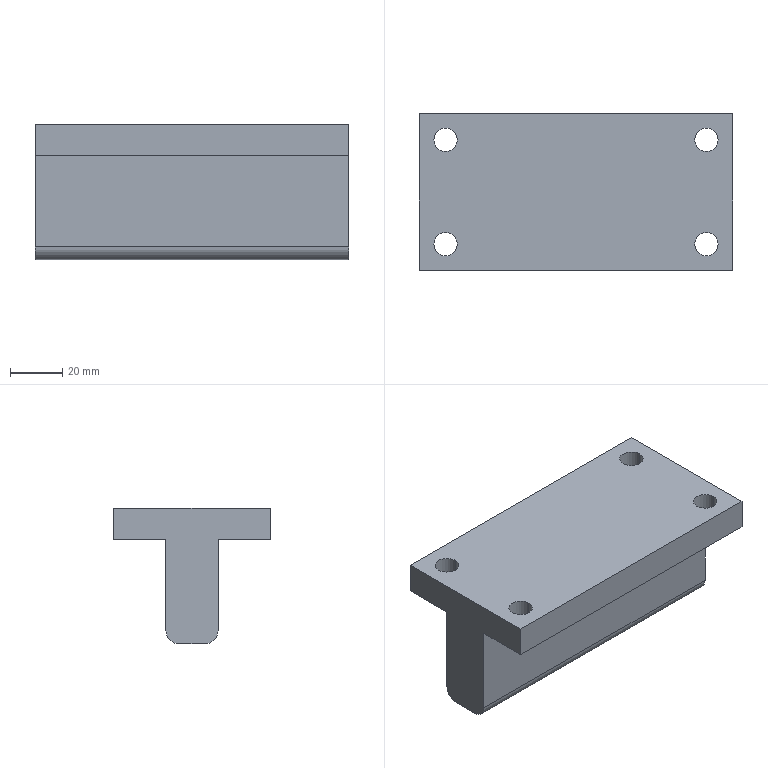Part | SolidWorks | features Extrusion 1, Fillet 1, HoleWzd 1, ICE 1 | 1 solid | 20 faces | box 120 x 60 x 52 mm | volume 178059 mm3 | cylinder 10 | plane 10 | commonest cylinder face diameters 9 x8 10 x2
STEP:
#1=CARTESIAN_POINT('',(114.5,50.,12.));
#2=VERTEX_POINT('',#1);
#3=CARTESIAN_POINT('',(105.5,50.,12.));
#4=VERTEX_POINT('',#3);
#5=CARTESIAN_POINT('',(110.,50.,12.));
#6=DIRECTION('',(0.,0.,-1.));
#7=DIRECTION('',(-1.,0.,0.));
#8=AXIS2_PLACEMENT_3D('',#5,#6,#7);
#9=CIRCLE('',#8,4.5);
#10=EDGE_CURVE('',#2,#4,#9,.T.);
#11=ORIENTED_EDGE('',*,*,#10,.F.);
#12=CARTESIAN_POINT('',(114.5,50.,0.));
#13=VERTEX_POINT('',#12);
#14=CARTESIAN_POINT('',(114.5,50.,0.));
#15=DIRECTION('',(0.,0.,-1.));
#16=VECTOR('',#15,1000.);
#17=LINE('',#14,#16);
#18=EDGE_CURVE('',#2,#13,#17,.T.);
#19=ORIENTED_EDGE('',*,*,#18,.T.);
#20=CARTESIAN_POINT('',(105.5,50.,0.));
#21=VERTEX_POINT('',#20);
#22=CARTESIAN_POINT('',(110.,50.,0.));
#23=DIRECTION('',(0.,0.,-1.));
#24=DIRECTION('',(-1.,0.,0.));
#25=AXIS2_PLACEMENT_3D('',#22,#23,#24);
#26=CIRCLE('',#25,4.5);
#27=EDGE_CURVE('',#13,#21,#26,.T.);
#28=ORIENTED_EDGE('',*,*,#27,.T.);
#29=CARTESIAN_POINT('',(105.5,50.,0.));
#30=DIRECTION('',(0.,0.,-1.));
#31=VECTOR('',#30,1000.);
#32=LINE('',#29,#31);
#33=EDGE_CURVE('',#4,#21,#32,.T.);
#34=ORIENTED_EDGE('',*,*,#33,.F.);
#35=EDGE_LOOP('',(#11,#19,#28,#34));
#36=FACE_OUTER_BOUND('',#35,.T.);
#37=CARTESIAN_POINT('',(110.,50.,0.));
#38=DIRECTION('',(0.,0.,-1.));
#39=DIRECTION('',(-1.,0.,0.));
#40=AXIS2_PLACEMENT_3D('',#37,#38,#39);
#41=CYLINDRICAL_SURFACE('',#40,4.5);
#42=ADVANCED_FACE('',(#36),#41,.F.);
#43=CARTESIAN_POINT('',(14.5,50.,12.));
#44=VERTEX_POINT('',#43);
#45=CARTESIAN_POINT('',(5.5,50.,12.));
#46=VERTEX_POINT('',#45);
#47=CARTESIAN_POINT('',(10.,50.,12.));
#48=DIRECTION('',(0.,0.,-1.));
#49=DIRECTION('',(-1.,0.,0.));
#50=AXIS2_PLACEMENT_3D('',#47,#48,#49);
#51=CIRCLE('',#50,4.5);
#52=EDGE_CURVE('',#44,#46,#51,.T.);
#53=ORIENTED_EDGE('',*,*,#52,.F.);
#54=CARTESIAN_POINT('',(14.5,50.,0.));
#55=VERTEX_POINT('',#54);
#56=CARTESIAN_POINT('',(14.5,50.,0.));
#57=DIRECTION('',(0.,0.,-1.));
#58=VECTOR('',#57,1000.);
#59=LINE('',#56,#58);
#60=EDGE_CURVE('',#44,#55,#59,.T.);
#61=ORIENTED_EDGE('',*,*,#60,.T.);
#62=CARTESIAN_POINT('',(5.5,50.,0.));
#63=VERTEX_POINT('',#62);
#64=CARTESIAN_POINT('',(10.,50.,0.));
#65=DIRECTION('',(0.,0.,-1.));
#66=DIRECTION('',(-1.,0.,0.));
#67=AXIS2_PLACEMENT_3D('',#64,#65,#66);
#68=CIRCLE('',#67,4.5);
#69=EDGE_CURVE('',#55,#63,#68,.T.);
#70=ORIENTED_EDGE('',*,*,#69,.T.);
#71=CARTESIAN_POINT('',(5.5,50.,0.));
#72=DIRECTION('',(0.,0.,-1.));
#73=VECTOR('',#72,1000.);
#74=LINE('',#71,#73);
#75=EDGE_CURVE('',#46,#63,#74,.T.);
#76=ORIENTED_EDGE('',*,*,#75,.F.);
#77=EDGE_LOOP('',(#53,#61,#70,#76));
#78=FACE_OUTER_BOUND('',#77,.T.);
#79=CARTESIAN_POINT('',(10.,50.,0.));
#80=DIRECTION('',(0.,0.,-1.));
#81=DIRECTION('',(-1.,0.,0.));
#82=AXIS2_PLACEMENT_3D('',#79,#80,#81);
#83=CYLINDRICAL_SURFACE('',#82,4.5);
#84=ADVANCED_FACE('',(#78),#83,.F.);
#85=CARTESIAN_POINT('',(14.5,10.,12.));
#86=VERTEX_POINT('',#85);
#87=CARTESIAN_POINT('',(5.5,10.,12.));
#88=VERTEX_POINT('',#87);
#89=CARTESIAN_POINT('',(10.,10.,12.));
#90=DIRECTION('',(0.,0.,-1.));
#91=DIRECTION('',(-1.,0.,0.));
#92=AXIS2_PLACEMENT_3D('',#89,#90,#91);
#93=CIRCLE('',#92,4.5);
#94=EDGE_CURVE('',#86,#88,#93,.T.);
#95=ORIENTED_EDGE('',*,*,#94,.F.);
#96=CARTESIAN_POINT('',(14.5,10.,0.));
#97=VERTEX_POINT('',#96);
#98=CARTESIAN_POINT('',(14.5,10.,0.));
#99=DIRECTION('',(0.,0.,-1.));
#100=VECTOR('',#99,1000.);
#101=LINE('',#98,#100);
#102=EDGE_CURVE('',#86,#97,#101,.T.);
#103=ORIENTED_EDGE('',*,*,#102,.T.);
#104=CARTESIAN_POINT('',(5.5,10.,0.));
#105=VERTEX_POINT('',#104);
#106=CARTESIAN_POINT('',(10.,10.,0.));
#107=DIRECTION('',(0.,0.,-1.));
#108=DIRECTION('',(-1.,0.,0.));
#109=AXIS2_PLACEMENT_3D('',#106,#107,#108);
#110=CIRCLE('',#109,4.5);
#111=EDGE_CURVE('',#97,#105,#110,.T.);
#112=ORIENTED_EDGE('',*,*,#111,.T.);
#113=CARTESIAN_POINT('',(5.5,10.,0.));
#114=DIRECTION('',(0.,0.,-1.));
#115=VECTOR('',#114,1000.);
#116=LINE('',#113,#115);
#117=EDGE_CURVE('',#88,#105,#116,.T.);
#118=ORIENTED_EDGE('',*,*,#117,.F.);
#119=EDGE_LOOP('',(#95,#103,#112,#118));
#120=FACE_OUTER_BOUND('',#119,.T.);
#121=CARTESIAN_POINT('',(10.,10.,0.));
#122=DIRECTION('',(0.,0.,-1.));
#123=DIRECTION('',(-1.,0.,0.));
#124=AXIS2_PLACEMENT_3D('',#121,#122,#123);
#125=CYLINDRICAL_SURFACE('',#124,4.5);
#126=ADVANCED_FACE('',(#120),#125,.F.);
#127=CARTESIAN_POINT('',(114.5,10.,12.));
#128=VERTEX_POINT('',#127);
#129=CARTESIAN_POINT('',(105.5,10.,12.));
#130=VERTEX_POINT('',#129);
#131=CARTESIAN_POINT('',(110.,10.,12.));
#132=DIRECTION('',(0.,0.,-1.));
#133=DIRECTION('',(-1.,0.,0.));
#134=AXIS2_PLACEMENT_3D('',#131,#132,#133);
#135=CIRCLE('',#134,4.5);
#136=EDGE_CURVE('',#128,#130,#135,.T.);
#137=ORIENTED_EDGE('',*,*,#136,.F.);
#138=CARTESIAN_POINT('',(114.5,10.,0.));
#139=VERTEX_POINT('',#138);
#140=CARTESIAN_POINT('',(114.5,10.,0.));
#141=DIRECTION('',(0.,0.,-1.));
#142=VECTOR('',#141,1000.);
#143=LINE('',#140,#142);
#144=EDGE_CURVE('',#128,#139,#143,.T.);
#145=ORIENTED_EDGE('',*,*,#144,.T.);
#146=CARTESIAN_POINT('',(105.5,10.,0.));
#147=VERTEX_POINT('',#146);
#148=CARTESIAN_POINT('',(110.,10.,0.));
#149=DIRECTION('',(0.,0.,-1.));
#150=DIRECTION('',(-1.,0.,0.));
#151=AXIS2_PLACEMENT_3D('',#148,#149,#150);
#152=CIRCLE('',#151,4.5);
#153=EDGE_CURVE('',#139,#147,#152,.T.);
#154=ORIENTED_EDGE('',*,*,#153,.T.);
#155=CARTESIAN_POINT('',(105.5,10.,0.));
#156=DIRECTION('',(0.,0.,-1.));
#157=VECTOR('',#156,1000.);
#158=LINE('',#155,#157);
#159=EDGE_CURVE('',#130,#147,#158,.T.);
#160=ORIENTED_EDGE('',*,*,#159,.F.);
#161=EDGE_LOOP('',(#137,#145,#154,#160));
#162=FACE_OUTER_BOUND('',#161,.T.);
#163=CARTESIAN_POINT('',(110.,10.,0.));
#164=DIRECTION('',(0.,0.,-1.));
#165=DIRECTION('',(-1.,0.,0.));
#166=AXIS2_PLACEMENT_3D('',#163,#164,#165);
#167=CYLINDRICAL_SURFACE('',#166,4.5);
#168=ADVANCED_FACE('',(#162),#167,.F.);
#169=CARTESIAN_POINT('',(110.,50.,0.));
#170=DIRECTION('',(0.,0.,-1.));
#171=DIRECTION('',(-1.,0.,0.));
#172=AXIS2_PLACEMENT_3D('',#169,#170,#171);
#173=CIRCLE('',#172,4.5);
#174=EDGE_CURVE('',#21,#13,#173,.T.);
#175=ORIENTED_EDGE('',*,*,#174,.F.);
#176=ORIENTED_EDGE('',*,*,#27,.F.);
#177=EDGE_LOOP('',(#175,#176));
#178=FACE_BOUND('',#177,.T.);
#179=CARTESIAN_POINT('',(10.,50.,0.));
#180=DIRECTION('',(0.,0.,-1.));
#181=DIRECTION('',(-1.,0.,0.));
#182=AXIS2_PLACEMENT_3D('',#179,#180,#181);
#183=CIRCLE('',#182,4.5);
#184=EDGE_CURVE('',#63,#55,#183,.T.);
#185=ORIENTED_EDGE('',*,*,#184,.F.);
#186=ORIENTED_EDGE('',*,*,#69,.F.);
#187=EDGE_LOOP('',(#185,#186));
#188=FACE_BOUND('',#187,.T.);
#189=CARTESIAN_POINT('',(120.,40.,0.));
#190=VERTEX_POINT('',#189);
#191=CARTESIAN_POINT('',(120.,60.,0.));
#192=VERTEX_POINT('',#191);
#193=CARTESIAN_POINT('',(120.,0.,0.));
#194=DIRECTION('',(0.,1.,0.));
#195=VECTOR('',#194,1000.);
#196=LINE('',#193,#195);
#197=EDGE_CURVE('',#190,#192,#196,.T.);
#198=ORIENTED_EDGE('',*,*,#197,.F.);
#199=CARTESIAN_POINT('',(0.,40.,0.));
#200=VERTEX_POINT('',#199);
#201=CARTESIAN_POINT('',(0.,40.,0.));
#202=DIRECTION('',(-1.,0.,0.));
#203=VECTOR('',#202,1000.);
#204=LINE('',#201,#203);
#205=EDGE_CURVE('',#190,#200,#204,.T.);
#206=ORIENTED_EDGE('',*,*,#205,.T.);
#207=CARTESIAN_POINT('',(0.,60.,0.));
#208=VERTEX_POINT('',#207);
#209=CARTESIAN_POINT('',(0.,0.,0.));
#210=DIRECTION('',(0.,1.,0.));
#211=VECTOR('',#210,1000.);
#212=LINE('',#209,#211);
#213=EDGE_CURVE('',#200,#208,#212,.T.);
#214=ORIENTED_EDGE('',*,*,#213,.T.);
#215=CARTESIAN_POINT('',(0.,60.,0.));
#216=DIRECTION('',(1.,0.,0.));
#217=VECTOR('',#216,1000.);
#218=LINE('',#215,#217);
#219=EDGE_CURVE('',#208,#192,#218,.T.);
#220=ORIENTED_EDGE('',*,*,#219,.T.);
#221=EDGE_LOOP('',(#198,#206,#214,#220));
#222=FACE_OUTER_BOUND('',#221,.T.);
#223=CARTESIAN_POINT('',(0.,0.,0.));
#224=DIRECTION('',(0.,0.,-1.));
#225=DIRECTION('',(-1.,0.,0.));
#226=AXIS2_PLACEMENT_3D('',#223,#224,#225);
#227=PLANE('',#226);
#228=ADVANCED_FACE('',(#178,#188,#222),#227,.T.);
#229=CARTESIAN_POINT('',(110.,10.,0.));
#230=DIRECTION('',(0.,0.,-1.));
#231=DIRECTION('',(-1.,0.,0.));
#232=AXIS2_PLACEMENT_3D('',#229,#230,#231);
#233=CIRCLE('',#232,4.5);
#234=EDGE_CURVE('',#147,#139,#233,.T.);
#235=ORIENTED_EDGE('',*,*,#234,.F.);
#236=ORIENTED_EDGE('',*,*,#153,.F.);
#237=EDGE_LOOP('',(#235,#236));
#238=FACE_BOUND('',#237,.T.);
#239=CARTESIAN_POINT('',(10.,10.,0.));
#240=DIRECTION('',(0.,0.,-1.));
#241=DIRECTION('',(-1.,0.,0.));
#242=AXIS2_PLACEMENT_3D('',#239,#240,#241);
#243=CIRCLE('',#242,4.5);
#244=EDGE_CURVE('',#105,#97,#243,.T.);
#245=ORIENTED_EDGE('',*,*,#244,.F.);
#246=ORIENTED_EDGE('',*,*,#111,.F.);
#247=EDGE_LOOP('',(#245,#246));
#248=FACE_BOUND('',#247,.T.);
#249=CARTESIAN_POINT('',(0.,0.,0.));
#250=VERTEX_POINT('',#249);
#251=CARTESIAN_POINT('',(0.,20.,0.));
#252=VERTEX_POINT('',#251);
#253=CARTESIAN_POINT('',(0.,0.,0.));
#254=DIRECTION('',(0.,1.,0.));
#255=VECTOR('',#254,1000.);
#256=LINE('',#253,#255);
#257=EDGE_CURVE('',#250,#252,#256,.T.);
#258=ORIENTED_EDGE('',*,*,#257,.T.);
#259=CARTESIAN_POINT('',(120.,20.,0.));
#260=VERTEX_POINT('',#259);
#261=CARTESIAN_POINT('',(0.,20.,0.));
#262=DIRECTION('',(1.,0.,0.));
#263=VECTOR('',#262,1000.);
#264=LINE('',#261,#263);
#265=EDGE_CURVE('',#252,#260,#264,.T.);
#266=ORIENTED_EDGE('',*,*,#265,.T.);
#267=CARTESIAN_POINT('',(120.,0.,0.));
#268=VERTEX_POINT('',#267);
#269=CARTESIAN_POINT('',(120.,0.,0.));
#270=DIRECTION('',(0.,1.,0.));
#271=VECTOR('',#270,1000.);
#272=LINE('',#269,#271);
#273=EDGE_CURVE('',#268,#260,#272,.T.);
#274=ORIENTED_EDGE('',*,*,#273,.F.);
#275=CARTESIAN_POINT('',(0.,0.,0.));
#276=DIRECTION('',(1.,0.,0.));
#277=VECTOR('',#276,1000.);
#278=LINE('',#275,#277);
#279=EDGE_CURVE('',#250,#268,#278,.T.);
#280=ORIENTED_EDGE('',*,*,#279,.F.);
#281=EDGE_LOOP('',(#258,#266,#274,#280));
#282=FACE_OUTER_BOUND('',#281,.T.);
#283=CARTESIAN_POINT('',(0.,0.,0.));
#284=DIRECTION('',(0.,0.,-1.));
#285=DIRECTION('',(-1.,0.,0.));
#286=AXIS2_PLACEMENT_3D('',#283,#284,#285);
#287=PLANE('',#286);
#288=ADVANCED_FACE('',(#238,#248,#282),#287,.T.);
#289=CARTESIAN_POINT('',(0.,40.,-35.));
#290=VERTEX_POINT('',#289);
#291=CARTESIAN_POINT('',(0.,40.,-40.));
#292=DIRECTION('',(0.,0.,1.));
#293=VECTOR('',#292,1000.);
#294=LINE('',#291,#293);
#295=EDGE_CURVE('',#290,#200,#294,.T.);
#296=ORIENTED_EDGE('',*,*,#295,.F.);
#297=CARTESIAN_POINT('',(0.,35.,-40.));
#298=VERTEX_POINT('',#297);
#299=CARTESIAN_POINT('',(0.,35.,-35.));
#300=DIRECTION('',(-1.,0.,0.));
#301=DIRECTION('',(0.,0.,1.));
#302=AXIS2_PLACEMENT_3D('',#299,#300,#301);
#303=CIRCLE('',#302,5.);
#304=EDGE_CURVE('',#290,#298,#303,.T.);
#305=ORIENTED_EDGE('',*,*,#304,.T.);
#306=CARTESIAN_POINT('',(0.,25.,-40.));
#307=VERTEX_POINT('',#306);
#308=CARTESIAN_POINT('',(0.,40.,-40.));
#309=DIRECTION('',(0.,-1.,0.));
#310=VECTOR('',#309,1000.);
#311=LINE('',#308,#310);
#312=EDGE_CURVE('',#298,#307,#311,.T.);
#313=ORIENTED_EDGE('',*,*,#312,.T.);
#314=CARTESIAN_POINT('',(0.,20.,-35.));
#315=VERTEX_POINT('',#314);
#316=CARTESIAN_POINT('',(0.,25.,-35.));
#317=DIRECTION('',(-1.,0.,0.));
#318=DIRECTION('',(0.,0.,1.));
#319=AXIS2_PLACEMENT_3D('',#316,#317,#318);
#320=CIRCLE('',#319,5.);
#321=EDGE_CURVE('',#307,#315,#320,.T.);
#322=ORIENTED_EDGE('',*,*,#321,.T.);
#323=CARTESIAN_POINT('',(0.,20.,-40.));
#324=DIRECTION('',(0.,0.,1.));
#325=VECTOR('',#324,1000.);
#326=LINE('',#323,#325);
#327=EDGE_CURVE('',#315,#252,#326,.T.);
#328=ORIENTED_EDGE('',*,*,#327,.T.);
#329=ORIENTED_EDGE('',*,*,#257,.F.);
#330=CARTESIAN_POINT('',(0.,0.,12.));
#331=VERTEX_POINT('',#330);
#332=CARTESIAN_POINT('',(0.,0.,12.));
#333=DIRECTION('',(0.,0.,-1.));
#334=VECTOR('',#333,1000.);
#335=LINE('',#332,#334);
#336=EDGE_CURVE('',#331,#250,#335,.T.);
#337=ORIENTED_EDGE('',*,*,#336,.F.);
#338=CARTESIAN_POINT('',(0.,60.,12.));
#339=VERTEX_POINT('',#338);
#340=CARTESIAN_POINT('',(0.,0.,12.));
#341=DIRECTION('',(0.,1.,0.));
#342=VECTOR('',#341,1000.);
#343=LINE('',#340,#342);
#344=EDGE_CURVE('',#331,#339,#343,.T.);
#345=ORIENTED_EDGE('',*,*,#344,.T.);
#346=CARTESIAN_POINT('',(0.,60.,12.));
#347=DIRECTION('',(0.,0.,-1.));
#348=VECTOR('',#347,1000.);
#349=LINE('',#346,#348);
#350=EDGE_CURVE('',#339,#208,#349,.T.);
#351=ORIENTED_EDGE('',*,*,#350,.T.);
#352=ORIENTED_EDGE('',*,*,#213,.F.);
#353=EDGE_LOOP('',(#296,#305,#313,#322,#328,#329,#337,#345,#351,#352));
#354=FACE_OUTER_BOUND('',#353,.T.);
#355=CARTESIAN_POINT('',(0.,0.,12.));
#356=DIRECTION('',(-1.,0.,0.));
#357=DIRECTION('',(0.,0.,1.));
#358=AXIS2_PLACEMENT_3D('',#355,#356,#357);
#359=PLANE('',#358);
#360=ADVANCED_FACE('',(#354),#359,.T.);
#361=ORIENTED_EDGE('',*,*,#279,.T.);
#362=CARTESIAN_POINT('',(120.,0.,12.));
#363=VERTEX_POINT('',#362);
#364=CARTESIAN_POINT('',(120.,0.,12.));
#365=DIRECTION('',(0.,0.,-1.));
#366=VECTOR('',#365,1000.);
#367=LINE('',#364,#366);
#368=EDGE_CURVE('',#363,#268,#367,.T.);
#369=ORIENTED_EDGE('',*,*,#368,.F.);
#370=CARTESIAN_POINT('',(0.,0.,12.));
#371=DIRECTION('',(1.,0.,0.));
#372=VECTOR('',#371,1000.);
#373=LINE('',#370,#372);
#374=EDGE_CURVE('',#331,#363,#373,.T.);
#375=ORIENTED_EDGE('',*,*,#374,.F.);
#376=ORIENTED_EDGE('',*,*,#336,.T.);
#377=EDGE_LOOP('',(#361,#369,#375,#376));
#378=FACE_OUTER_BOUND('',#377,.T.);
#379=CARTESIAN_POINT('',(0.,0.,12.));
#380=DIRECTION('',(0.,1.,0.));
#381=DIRECTION('',(0.,0.,1.));
#382=AXIS2_PLACEMENT_3D('',#379,#380,#381);
#383=PLANE('',#382);
#384=ADVANCED_FACE('',(#378),#383,.F.);
#385=CARTESIAN_POINT('',(120.,25.,-40.));
#386=VERTEX_POINT('',#385);
#387=CARTESIAN_POINT('',(120.,35.,-40.));
#388=VERTEX_POINT('',#387);
#389=CARTESIAN_POINT('',(120.,40.,-40.));
#390=DIRECTION('',(0.,1.,0.));
#391=VECTOR('',#390,1000.);
#392=LINE('',#389,#391);
#393=EDGE_CURVE('',#386,#388,#392,.T.);
#394=ORIENTED_EDGE('',*,*,#393,.T.);
#395=CARTESIAN_POINT('',(120.,40.,-35.));
#396=VERTEX_POINT('',#395);
#397=CARTESIAN_POINT('',(120.,35.,-35.));
#398=DIRECTION('',(1.,0.,0.));
#399=DIRECTION('',(0.,0.,1.));
#400=AXIS2_PLACEMENT_3D('',#397,#398,#399);
#401=CIRCLE('',#400,5.);
#402=EDGE_CURVE('',#388,#396,#401,.T.);
#403=ORIENTED_EDGE('',*,*,#402,.T.);
#404=CARTESIAN_POINT('',(120.,40.,-40.));
#405=DIRECTION('',(0.,0.,1.));
#406=VECTOR('',#405,1000.);
#407=LINE('',#404,#406);
#408=EDGE_CURVE('',#396,#190,#407,.T.);
#409=ORIENTED_EDGE('',*,*,#408,.T.);
#410=ORIENTED_EDGE('',*,*,#197,.T.);
#411=CARTESIAN_POINT('',(120.,60.,12.));
#412=VERTEX_POINT('',#411);
#413=CARTESIAN_POINT('',(120.,60.,12.));
#414=DIRECTION('',(0.,0.,-1.));
#415=VECTOR('',#414,1000.);
#416=LINE('',#413,#415);
#417=EDGE_CURVE('',#412,#192,#416,.T.);
#418=ORIENTED_EDGE('',*,*,#417,.F.);
#419=CARTESIAN_POINT('',(120.,0.,12.));
#420=DIRECTION('',(0.,1.,0.));
#421=VECTOR('',#420,1000.);
#422=LINE('',#419,#421);
#423=EDGE_CURVE('',#363,#412,#422,.T.);
#424=ORIENTED_EDGE('',*,*,#423,.F.);
#425=ORIENTED_EDGE('',*,*,#368,.T.);
#426=ORIENTED_EDGE('',*,*,#273,.T.);
#427=CARTESIAN_POINT('',(120.,20.,-35.));
#428=VERTEX_POINT('',#427);
#429=CARTESIAN_POINT('',(120.,20.,-40.));
#430=DIRECTION('',(0.,0.,1.));
#431=VECTOR('',#430,1000.);
#432=LINE('',#429,#431);
#433=EDGE_CURVE('',#428,#260,#432,.T.);
#434=ORIENTED_EDGE('',*,*,#433,.F.);
#435=CARTESIAN_POINT('',(120.,25.,-35.));
#436=DIRECTION('',(1.,0.,0.));
#437=DIRECTION('',(0.,0.,1.));
#438=AXIS2_PLACEMENT_3D('',#435,#436,#437);
#439=CIRCLE('',#438,5.);
#440=EDGE_CURVE('',#428,#386,#439,.T.);
#441=ORIENTED_EDGE('',*,*,#440,.T.);
#442=EDGE_LOOP('',(#394,#403,#409,#410,#418,#424,#425,#426,#434,#441));
#443=FACE_OUTER_BOUND('',#442,.T.);
#444=CARTESIAN_POINT('',(120.,0.,12.));
#445=DIRECTION('',(-1.,0.,0.));
#446=DIRECTION('',(0.,0.,1.));
#447=AXIS2_PLACEMENT_3D('',#444,#445,#446);
#448=PLANE('',#447);
#449=ADVANCED_FACE('',(#443),#448,.F.);
#450=ORIENTED_EDGE('',*,*,#219,.F.);
#451=ORIENTED_EDGE('',*,*,#350,.F.);
#452=CARTESIAN_POINT('',(0.,60.,12.));
#453=DIRECTION('',(1.,0.,0.));
#454=VECTOR('',#453,1000.);
#455=LINE('',#452,#454);
#456=EDGE_CURVE('',#339,#412,#455,.T.);
#457=ORIENTED_EDGE('',*,*,#456,.T.);
#458=ORIENTED_EDGE('',*,*,#417,.T.);
#459=EDGE_LOOP('',(#450,#451,#457,#458));
#460=FACE_OUTER_BOUND('',#459,.T.);
#461=CARTESIAN_POINT('',(0.,60.,12.));
#462=DIRECTION('',(0.,1.,0.));
#463=DIRECTION('',(0.,0.,1.));
#464=AXIS2_PLACEMENT_3D('',#461,#462,#463);
#465=PLANE('',#464);
#466=ADVANCED_FACE('',(#460),#465,.T.);
#467=CARTESIAN_POINT('',(110.,50.,12.));
#468=DIRECTION('',(0.,0.,-1.));
#469=DIRECTION('',(-1.,0.,0.));
#470=AXIS2_PLACEMENT_3D('',#467,#468,#469);
#471=CIRCLE('',#470,4.5);
#472=EDGE_CURVE('',#4,#2,#471,.T.);
#473=ORIENTED_EDGE('',*,*,#472,.T.);
#474=ORIENTED_EDGE('',*,*,#10,.T.);
#475=EDGE_LOOP('',(#473,#474));
#476=FACE_BOUND('',#475,.T.);
#477=CARTESIAN_POINT('',(10.,50.,12.));
#478=DIRECTION('',(0.,0.,-1.));
#479=DIRECTION('',(-1.,0.,0.));
#480=AXIS2_PLACEMENT_3D('',#477,#478,#479);
#481=CIRCLE('',#480,4.5);
#482=EDGE_CURVE('',#46,#44,#481,.T.);
#483=ORIENTED_EDGE('',*,*,#482,.T.);
#484=ORIENTED_EDGE('',*,*,#52,.T.);
#485=EDGE_LOOP('',(#483,#484));
#486=FACE_BOUND('',#485,.T.);
#487=CARTESIAN_POINT('',(10.,10.,12.));
#488=DIRECTION('',(0.,0.,-1.));
#489=DIRECTION('',(-1.,0.,0.));
#490=AXIS2_PLACEMENT_3D('',#487,#488,#489);
#491=CIRCLE('',#490,4.5);
#492=EDGE_CURVE('',#88,#86,#491,.T.);
#493=ORIENTED_EDGE('',*,*,#492,.T.);
#494=ORIENTED_EDGE('',*,*,#94,.T.);
#495=EDGE_LOOP('',(#493,#494));
#496=FACE_BOUND('',#495,.T.);
#497=CARTESIAN_POINT('',(110.,10.,12.));
#498=DIRECTION('',(0.,0.,-1.));
#499=DIRECTION('',(-1.,0.,0.));
#500=AXIS2_PLACEMENT_3D('',#497,#498,#499);
#501=CIRCLE('',#500,4.5);
#502=EDGE_CURVE('',#130,#128,#501,.T.);
#503=ORIENTED_EDGE('',*,*,#502,.T.);
#504=ORIENTED_EDGE('',*,*,#136,.T.);
#505=EDGE_LOOP('',(#503,#504));
#506=FACE_BOUND('',#505,.T.);
#507=ORIENTED_EDGE('',*,*,#344,.F.);
#508=ORIENTED_EDGE('',*,*,#374,.T.);
#509=ORIENTED_EDGE('',*,*,#423,.T.);
#510=ORIENTED_EDGE('',*,*,#456,.F.);
#511=EDGE_LOOP('',(#507,#508,#509,#510));
#512=FACE_OUTER_BOUND('',#511,.T.);
#513=CARTESIAN_POINT('',(0.,0.,12.));
#514=DIRECTION('',(0.,0.,-1.));
#515=DIRECTION('',(-1.,0.,0.));
#516=AXIS2_PLACEMENT_3D('',#513,#514,#515);
#517=PLANE('',#516);
#518=ADVANCED_FACE('',(#476,#486,#496,#506,#512),#517,.F.);
#519=ORIENTED_EDGE('',*,*,#144,.F.);
#520=ORIENTED_EDGE('',*,*,#502,.F.);
#521=ORIENTED_EDGE('',*,*,#159,.T.);
#522=ORIENTED_EDGE('',*,*,#234,.T.);
#523=EDGE_LOOP('',(#519,#520,#521,#522));
#524=FACE_OUTER_BOUND('',#523,.T.);
#525=CARTESIAN_POINT('',(110.,10.,0.));
#526=DIRECTION('',(0.,0.,-1.));
#527=DIRECTION('',(-1.,0.,0.));
#528=AXIS2_PLACEMENT_3D('',#525,#526,#527);
#529=CYLINDRICAL_SURFACE('',#528,4.5);
#530=ADVANCED_FACE('',(#524),#529,.F.);
#531=ORIENTED_EDGE('',*,*,#102,.F.);
#532=ORIENTED_EDGE('',*,*,#492,.F.);
#533=ORIENTED_EDGE('',*,*,#117,.T.);
#534=ORIENTED_EDGE('',*,*,#244,.T.);
#535=EDGE_LOOP('',(#531,#532,#533,#534));
#536=FACE_OUTER_BOUND('',#535,.T.);
#537=CARTESIAN_POINT('',(10.,10.,0.));
#538=DIRECTION('',(0.,0.,-1.));
#539=DIRECTION('',(-1.,0.,0.));
#540=AXIS2_PLACEMENT_3D('',#537,#538,#539);
#541=CYLINDRICAL_SURFACE('',#540,4.5);
#542=ADVANCED_FACE('',(#536),#541,.F.);
#543=ORIENTED_EDGE('',*,*,#60,.F.);
#544=ORIENTED_EDGE('',*,*,#482,.F.);
#545=ORIENTED_EDGE('',*,*,#75,.T.);
#546=ORIENTED_EDGE('',*,*,#184,.T.);
#547=EDGE_LOOP('',(#543,#544,#545,#546));
#548=FACE_OUTER_BOUND('',#547,.T.);
#549=CARTESIAN_POINT('',(10.,50.,0.));
#550=DIRECTION('',(0.,0.,-1.));
#551=DIRECTION('',(-1.,0.,0.));
#552=AXIS2_PLACEMENT_3D('',#549,#550,#551);
#553=CYLINDRICAL_SURFACE('',#552,4.5);
#554=ADVANCED_FACE('',(#548),#553,.F.);
#555=ORIENTED_EDGE('',*,*,#18,.F.);
#556=ORIENTED_EDGE('',*,*,#472,.F.);
#557=ORIENTED_EDGE('',*,*,#33,.T.);
#558=ORIENTED_EDGE('',*,*,#174,.T.);
#559=EDGE_LOOP('',(#555,#556,#557,#558));
#560=FACE_OUTER_BOUND('',#559,.T.);
#561=CARTESIAN_POINT('',(110.,50.,0.));
#562=DIRECTION('',(0.,0.,-1.));
#563=DIRECTION('',(-1.,0.,0.));
#564=AXIS2_PLACEMENT_3D('',#561,#562,#563);
#565=CYLINDRICAL_SURFACE('',#564,4.5);
#566=ADVANCED_FACE('',(#560),#565,.F.);
#567=ORIENTED_EDGE('',*,*,#327,.F.);
#568=CARTESIAN_POINT('',(120.,20.,-35.));
#569=DIRECTION('',(1.,0.,0.));
#570=VECTOR('',#569,1000.);
#571=LINE('',#568,#570);
#572=EDGE_CURVE('',#315,#428,#571,.T.);
#573=ORIENTED_EDGE('',*,*,#572,.T.);
#574=ORIENTED_EDGE('',*,*,#433,.T.);
#575=ORIENTED_EDGE('',*,*,#265,.F.);
#576=EDGE_LOOP('',(#567,#573,#574,#575));
#577=FACE_OUTER_BOUND('',#576,.T.);
#578=CARTESIAN_POINT('',(0.,20.,-40.));
#579=DIRECTION('',(0.,-1.,0.));
#580=DIRECTION('',(0.,0.,-1.));
#581=AXIS2_PLACEMENT_3D('',#578,#579,#580);
#582=PLANE('',#581);
#583=ADVANCED_FACE('',(#577),#582,.T.);
#584=ORIENTED_EDGE('',*,*,#408,.F.);
#585=CARTESIAN_POINT('',(0.,40.,-35.));
#586=DIRECTION('',(-1.,0.,0.));
#587=VECTOR('',#586,1000.);
#588=LINE('',#585,#587);
#589=EDGE_CURVE('',#396,#290,#588,.T.);
#590=ORIENTED_EDGE('',*,*,#589,.T.);
#591=ORIENTED_EDGE('',*,*,#295,.T.);
#592=ORIENTED_EDGE('',*,*,#205,.F.);
#593=EDGE_LOOP('',(#584,#590,#591,#592));
#594=FACE_OUTER_BOUND('',#593,.T.);
#595=CARTESIAN_POINT('',(0.,40.,-40.));
#596=DIRECTION('',(0.,1.,0.));
#597=DIRECTION('',(0.,0.,1.));
#598=AXIS2_PLACEMENT_3D('',#595,#596,#597);
#599=PLANE('',#598);
#600=ADVANCED_FACE('',(#594),#599,.T.);
#601=ORIENTED_EDGE('',*,*,#312,.F.);
#602=CARTESIAN_POINT('',(120.,35.,-40.));
#603=DIRECTION('',(1.,0.,0.));
#604=VECTOR('',#603,1000.);
#605=LINE('',#602,#604);
#606=EDGE_CURVE('',#298,#388,#605,.T.);
#607=ORIENTED_EDGE('',*,*,#606,.T.);
#608=ORIENTED_EDGE('',*,*,#393,.F.);
#609=CARTESIAN_POINT('',(0.,25.,-40.));
#610=DIRECTION('',(-1.,0.,0.));
#611=VECTOR('',#610,1000.);
#612=LINE('',#609,#611);
#613=EDGE_CURVE('',#386,#307,#612,.T.);
#614=ORIENTED_EDGE('',*,*,#613,.T.);
#615=EDGE_LOOP('',(#601,#607,#608,#614));
#616=FACE_OUTER_BOUND('',#615,.T.);
#617=CARTESIAN_POINT('',(0.,0.,-40.));
#618=DIRECTION('',(0.,0.,1.));
#619=DIRECTION('',(1.,0.,0.));
#620=AXIS2_PLACEMENT_3D('',#617,#618,#619);
#621=PLANE('',#620);
#622=ADVANCED_FACE('',(#616),#621,.F.);
#623=ORIENTED_EDGE('',*,*,#402,.F.);
#624=ORIENTED_EDGE('',*,*,#606,.F.);
#625=ORIENTED_EDGE('',*,*,#304,.F.);
#626=ORIENTED_EDGE('',*,*,#589,.F.);
#627=EDGE_LOOP('',(#623,#624,#625,#626));
#628=FACE_OUTER_BOUND('',#627,.T.);
#629=CARTESIAN_POINT('',(0.,35.,-35.));
#630=DIRECTION('',(1.,0.,0.));
#631=DIRECTION('',(0.,0.,-1.));
#632=AXIS2_PLACEMENT_3D('',#629,#630,#631);
#633=CYLINDRICAL_SURFACE('',#632,5.);
#634=ADVANCED_FACE('',(#628),#633,.T.);
#635=ORIENTED_EDGE('',*,*,#321,.F.);
#636=ORIENTED_EDGE('',*,*,#613,.F.);
#637=ORIENTED_EDGE('',*,*,#440,.F.);
#638=ORIENTED_EDGE('',*,*,#572,.F.);
#639=EDGE_LOOP('',(#635,#636,#637,#638));
#640=FACE_OUTER_BOUND('',#639,.T.);
#641=CARTESIAN_POINT('',(0.,25.,-35.));
#642=DIRECTION('',(-1.,0.,0.));
#643=DIRECTION('',(0.,0.,1.));
#644=AXIS2_PLACEMENT_3D('',#641,#642,#643);
#645=CYLINDRICAL_SURFACE('',#644,5.);
#646=ADVANCED_FACE('',(#640),#645,.T.);
#647=CLOSED_SHELL('',(#42,#84,#126,#168,#228,#288,#360,#384,#449,#466,#518,#530,#542,#554,#566,#583,#600,#622,#634,#646));
#648=MANIFOLD_SOLID_BREP('',#647);
#649=CARTESIAN_POINT('',(0.,0.,0.));
#650=DIRECTION('',(0.,0.,1.));
#651=DIRECTION('',(1.,0.,0.));
#652=AXIS2_PLACEMENT_3D('',#649,#650,#651);
#653=(LENGTH_UNIT()NAMED_UNIT(*)SI_UNIT(.MILLI.,.METRE.));
#654=UNCERTAINTY_MEASURE_WITH_UNIT(LENGTH_MEASURE(0.00001),#653,'','');
#655=(NAMED_UNIT(*)PLANE_ANGLE_UNIT()SI_UNIT($,.RADIAN.));
#656=(NAMED_UNIT(*)SI_UNIT($,.STERADIAN.)SOLID_ANGLE_UNIT());
#657=(GEOMETRIC_REPRESENTATION_CONTEXT(3)GLOBAL_UNCERTAINTY_ASSIGNED_CONTEXT((#654))GLOBAL_UNIT_ASSIGNED_CONTEXT((#653,#655,#656))REPRESENTATION_CONTEXT('',''));
#658=ADVANCED_BREP_SHAPE_REPRESENTATION('',(#648,#652),#657);